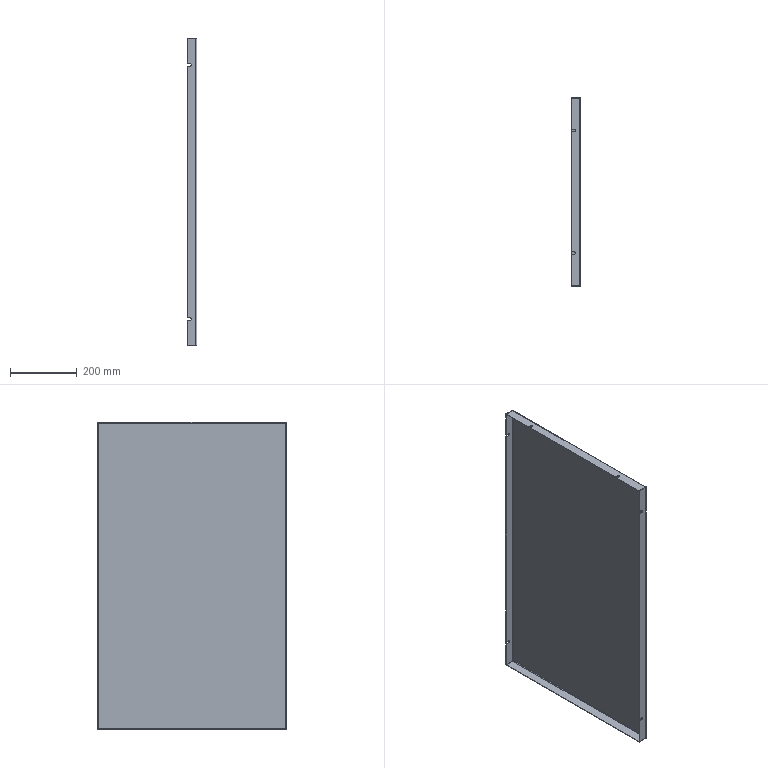Part | STEP file | SMEB-2 | 1 solid | 58 faces | box 30 x 568 x 923 mm | volume 908170 mm3 | plane 44 | cylinder 14 | commonest cylinder face diameters 7 x6 3 x4 6 x4